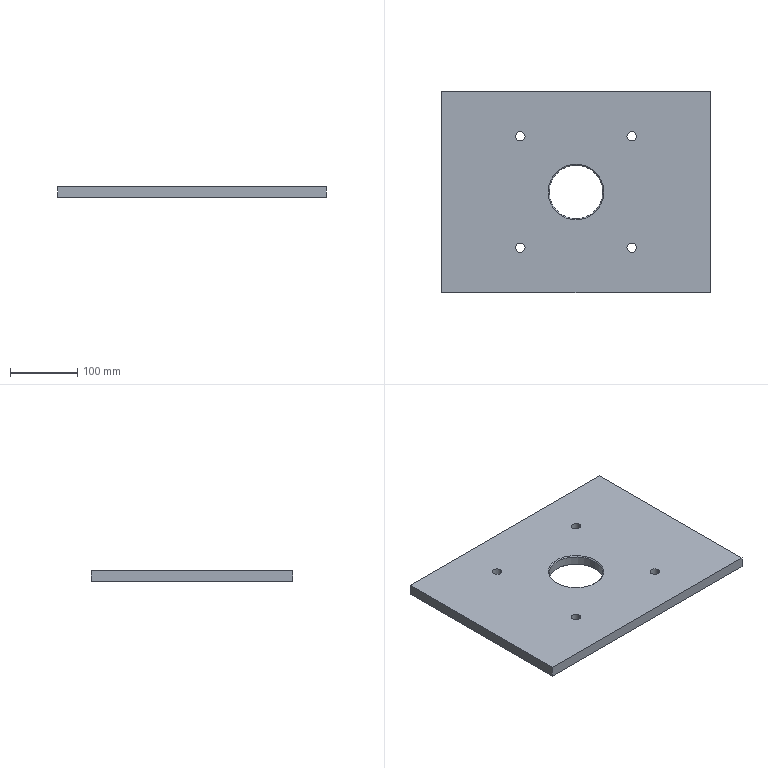Part | STEP file | 04-Base plate | 1 solid | 20 faces | box 400 x 300 x 16 mm | volume 1829151 mm3 | cylinder 10 | plane 6 | cone 4 | commonest cylinder face diameters 14 x8 80 x2
STEP:
#1=CARTESIAN_POINT('',(0.,0.,0.));
#2=DIRECTION('',(0.,0.,1.));
#3=DIRECTION('',(1.,0.,0.));
#4=AXIS2_PLACEMENT_3D('',#1,#2,#3);
#5=CARTESIAN_POINT('',(240.,-150.,14.5));
#6=VERTEX_POINT('',#5);
#7=CARTESIAN_POINT('',(241.5,-150.,16.));
#8=VERTEX_POINT('',#7);
#9=CARTESIAN_POINT('',(240.,-150.,14.5));
#10=DIRECTION('',(0.7071,0.,0.7071));
#11=VECTOR('',#10,1.);
#12=LINE('',#9,#11);
#13=CARTESIAN_POINT('',(200.,-150.,14.5));
#14=DIRECTION('',(0.,0.,1.));
#15=DIRECTION('',(1.,0.,0.));
#16=AXIS2_PLACEMENT_3D('',#13,#14,#15);
#17=CONICAL_SURFACE('',#16,40.,0.7854);
#18=CARTESIAN_POINT('',(6.283,0.));
#19=DIRECTION('',(0.,1.));
#20=VECTOR('',#19,1.);
#21=LINE('',#18,#20);
#22=(GEOMETRIC_REPRESENTATION_CONTEXT(2)PARAMETRIC_REPRESENTATION_CONTEXT()REPRESENTATION_CONTEXT('',''));
#23=DEFINITIONAL_REPRESENTATION('',(#21),#22);
#24=PCURVE('',#17,#23);
#25=CARTESIAN_POINT('',(200.,-150.,14.5));
#26=DIRECTION('',(0.,0.,1.));
#27=DIRECTION('',(1.,0.,0.));
#28=AXIS2_PLACEMENT_3D('',#25,#26,#27);
#29=CONICAL_SURFACE('',#28,40.,0.7854);
#30=CARTESIAN_POINT('',(0.,0.));
#31=DIRECTION('',(0.,1.));
#32=VECTOR('',#31,1.);
#33=LINE('',#30,#32);
#34=(GEOMETRIC_REPRESENTATION_CONTEXT(2)PARAMETRIC_REPRESENTATION_CONTEXT()REPRESENTATION_CONTEXT('',''));
#35=DEFINITIONAL_REPRESENTATION('',(#33),#34);
#36=PCURVE('',#29,#35);
#37=SURFACE_CURVE('',#12,(#24,#36),.PCURVE_S1.);
#38=EDGE_CURVE('',#6,#8,#37,.T.);
#39=ORIENTED_EDGE('',*,*,#38,.T.);
#40=CARTESIAN_POINT('',(158.5,-150.,16.));
#41=VERTEX_POINT('',#40);
#42=CARTESIAN_POINT('',(200.,-150.,16.));
#43=DIRECTION('',(0.,0.,-1.));
#44=DIRECTION('',(1.,0.,0.));
#45=AXIS2_PLACEMENT_3D('',#42,#43,#44);
#46=CIRCLE('',#45,41.5);
#47=CARTESIAN_POINT('',(6.283,1.5));
#48=DIRECTION('',(-1.,0.));
#49=VECTOR('',#48,1.);
#50=LINE('',#47,#49);
#51=(GEOMETRIC_REPRESENTATION_CONTEXT(2)PARAMETRIC_REPRESENTATION_CONTEXT()REPRESENTATION_CONTEXT('',''));
#52=DEFINITIONAL_REPRESENTATION('',(#50),#51);
#53=PCURVE('',#17,#52);
#54=CARTESIAN_POINT('',(0.,0.,16.));
#55=DIRECTION('',(0.,0.,1.));
#56=DIRECTION('',(1.,0.,0.));
#57=AXIS2_PLACEMENT_3D('',#54,#55,#56);
#58=PLANE('',#57);
#59=CARTESIAN_POINT('',(241.5,-150.));
#60=CARTESIAN_POINT('',(241.5,-221.88));
#61=CARTESIAN_POINT('',(179.25,-185.94));
#62=CARTESIAN_POINT('',(117.,-150.));
#63=CARTESIAN_POINT('',(179.25,-114.06));
#64=CARTESIAN_POINT('',(241.5,-78.12));
#65=CARTESIAN_POINT('',(241.5,-150.));
#66=(BOUNDED_CURVE()B_SPLINE_CURVE(2,(#59,#60,#61,#62,#63,#64,#65),.UNSPECIFIED.,.T.,.F.)B_SPLINE_CURVE_WITH_KNOTS((1,2,2,2,2,1),(-2.094,0.,2.094,4.189,6.283,8.378),.UNSPECIFIED.)CURVE()GEOMETRIC_REPRESENTATION_ITEM()RATIONAL_B_SPLINE_CURVE((1.,0.5,1.,0.5,1.,0.5,1.))REPRESENTATION_ITEM(''));
#67=(GEOMETRIC_REPRESENTATION_CONTEXT(2)PARAMETRIC_REPRESENTATION_CONTEXT()REPRESENTATION_CONTEXT('',''));
#68=DEFINITIONAL_REPRESENTATION('',(#66),#67);
#69=PCURVE('',#58,#68);
#70=SURFACE_CURVE('',#46,(#53,#69),.PCURVE_S1.);
#71=EDGE_CURVE('',#8,#41,#70,.T.);
#72=ORIENTED_EDGE('',*,*,#71,.T.);
#73=CARTESIAN_POINT('',(160.,-150.,14.5));
#74=VERTEX_POINT('',#73);
#75=CARTESIAN_POINT('',(160.,-150.,14.5));
#76=DIRECTION('',(-0.7071,0.,0.7071));
#77=VECTOR('',#76,1.);
#78=LINE('',#75,#77);
#79=CARTESIAN_POINT('',(3.142,0.));
#80=DIRECTION('',(0.,1.));
#81=VECTOR('',#80,1.);
#82=LINE('',#79,#81);
#83=(GEOMETRIC_REPRESENTATION_CONTEXT(2)PARAMETRIC_REPRESENTATION_CONTEXT()REPRESENTATION_CONTEXT('',''));
#84=DEFINITIONAL_REPRESENTATION('',(#82),#83);
#85=PCURVE('',#17,#84);
#86=CARTESIAN_POINT('',(3.142,0.));
#87=DIRECTION('',(0.,1.));
#88=VECTOR('',#87,1.);
#89=LINE('',#86,#88);
#90=(GEOMETRIC_REPRESENTATION_CONTEXT(2)PARAMETRIC_REPRESENTATION_CONTEXT()REPRESENTATION_CONTEXT('',''));
#91=DEFINITIONAL_REPRESENTATION('',(#89),#90);
#92=PCURVE('',#29,#91);
#93=SURFACE_CURVE('',#78,(#85,#92),.PCURVE_S1.);
#94=EDGE_CURVE('',#74,#41,#93,.T.);
#95=ORIENTED_EDGE('',*,*,#94,.F.);
#96=CARTESIAN_POINT('',(200.,-150.,14.5));
#97=DIRECTION('',(0.,0.,1.));
#98=DIRECTION('',(1.,0.,0.));
#99=AXIS2_PLACEMENT_3D('',#96,#97,#98);
#100=CIRCLE('',#99,40.);
#101=CARTESIAN_POINT('',(0.,0.));
#102=DIRECTION('',(1.,0.));
#103=VECTOR('',#102,1.);
#104=LINE('',#101,#103);
#105=(GEOMETRIC_REPRESENTATION_CONTEXT(2)PARAMETRIC_REPRESENTATION_CONTEXT()REPRESENTATION_CONTEXT('',''));
#106=DEFINITIONAL_REPRESENTATION('',(#104),#105);
#107=PCURVE('',#17,#106);
#108=CARTESIAN_POINT('',(200.,-150.,16.));
#109=DIRECTION('',(0.,0.,-1.));
#110=DIRECTION('',(-1.,0.,0.));
#111=AXIS2_PLACEMENT_3D('',#108,#109,#110);
#112=CYLINDRICAL_SURFACE('',#111,40.);
#113=CARTESIAN_POINT('',(9.425,1.5));
#114=DIRECTION('',(-1.,0.));
#115=VECTOR('',#114,1.);
#116=LINE('',#113,#115);
#117=(GEOMETRIC_REPRESENTATION_CONTEXT(2)PARAMETRIC_REPRESENTATION_CONTEXT()REPRESENTATION_CONTEXT('',''));
#118=DEFINITIONAL_REPRESENTATION('',(#116),#117);
#119=PCURVE('',#112,#118);
#120=SURFACE_CURVE('',#100,(#107,#119),.PCURVE_S1.);
#121=EDGE_CURVE('',#74,#6,#120,.T.);
#122=ORIENTED_EDGE('',*,*,#121,.T.);
#123=EDGE_LOOP('',(#39,#72,#95,#122));
#124=FACE_BOUND('',#123,.F.);
#125=ADVANCED_FACE('',(#124),#17,.F.);
#126=CARTESIAN_POINT('',(160.,-150.,1.5));
#127=VERTEX_POINT('',#126);
#128=CARTESIAN_POINT('',(158.5,-150.,0.));
#129=VERTEX_POINT('',#128);
#130=CARTESIAN_POINT('',(158.5,-150.,0.));
#131=DIRECTION('',(-0.7071,0.,-0.7071));
#132=VECTOR('',#131,1.);
#133=LINE('',#130,#132);
#134=CARTESIAN_POINT('',(200.,-150.,0.));
#135=DIRECTION('',(0.,0.,-1.));
#136=DIRECTION('',(-1.,0.,0.));
#137=AXIS2_PLACEMENT_3D('',#134,#135,#136);
#138=CONICAL_SURFACE('',#137,41.5,0.7854);
#139=CARTESIAN_POINT('',(6.283,0.));
#140=DIRECTION('',(0.,1.));
#141=VECTOR('',#140,1.);
#142=LINE('',#139,#141);
#143=(GEOMETRIC_REPRESENTATION_CONTEXT(2)PARAMETRIC_REPRESENTATION_CONTEXT()REPRESENTATION_CONTEXT('',''));
#144=DEFINITIONAL_REPRESENTATION('',(#142),#143);
#145=PCURVE('',#138,#144);
#146=CARTESIAN_POINT('',(200.,-150.,0.));
#147=DIRECTION('',(0.,0.,-1.));
#148=DIRECTION('',(-1.,0.,0.));
#149=AXIS2_PLACEMENT_3D('',#146,#147,#148);
#150=CONICAL_SURFACE('',#149,41.5,0.7854);
#151=CARTESIAN_POINT('',(0.,0.));
#152=DIRECTION('',(0.,1.));
#153=VECTOR('',#152,1.);
#154=LINE('',#151,#153);
#155=(GEOMETRIC_REPRESENTATION_CONTEXT(2)PARAMETRIC_REPRESENTATION_CONTEXT()REPRESENTATION_CONTEXT('',''));
#156=DEFINITIONAL_REPRESENTATION('',(#154),#155);
#157=PCURVE('',#150,#156);
#158=SURFACE_CURVE('',#133,(#145,#157),.PCURVE_S1.);
#159=EDGE_CURVE('',#127,#129,#158,.T.);
#160=ORIENTED_EDGE('',*,*,#159,.T.);
#161=CARTESIAN_POINT('',(241.5,-150.,0.));
#162=VERTEX_POINT('',#161);
#163=CARTESIAN_POINT('',(200.,-150.,0.));
#164=DIRECTION('',(0.,0.,1.));
#165=DIRECTION('',(1.,0.,0.));
#166=AXIS2_PLACEMENT_3D('',#163,#164,#165);
#167=CIRCLE('',#166,41.5);
#168=CARTESIAN_POINT('',(9.425,0.));
#169=DIRECTION('',(-1.,0.));
#170=VECTOR('',#169,1.);
#171=LINE('',#168,#170);
#172=(GEOMETRIC_REPRESENTATION_CONTEXT(2)PARAMETRIC_REPRESENTATION_CONTEXT()REPRESENTATION_CONTEXT('',''));
#173=DEFINITIONAL_REPRESENTATION('',(#171),#172);
#174=PCURVE('',#138,#173);
#175=CARTESIAN_POINT('',(0.,0.,0.));
#176=DIRECTION('',(0.,0.,1.));
#177=DIRECTION('',(1.,0.,0.));
#178=AXIS2_PLACEMENT_3D('',#175,#176,#177);
#179=PLANE('',#178);
#180=CARTESIAN_POINT('',(200.,-150.));
#181=DIRECTION('',(1.,0.));
#182=AXIS2_PLACEMENT_2D('',#180,#181);
#183=CIRCLE('',#182,41.5);
#184=(GEOMETRIC_REPRESENTATION_CONTEXT(2)PARAMETRIC_REPRESENTATION_CONTEXT()REPRESENTATION_CONTEXT('',''));
#185=DEFINITIONAL_REPRESENTATION('',(#183),#184);
#186=PCURVE('',#179,#185);
#187=SURFACE_CURVE('',#167,(#174,#186),.PCURVE_S1.);
#188=EDGE_CURVE('',#129,#162,#187,.T.);
#189=ORIENTED_EDGE('',*,*,#188,.T.);
#190=CARTESIAN_POINT('',(240.,-150.,1.5));
#191=VERTEX_POINT('',#190);
#192=CARTESIAN_POINT('',(241.5,-150.,0.));
#193=DIRECTION('',(0.7071,0.,-0.7071));
#194=VECTOR('',#193,1.);
#195=LINE('',#192,#194);
#196=CARTESIAN_POINT('',(3.142,0.));
#197=DIRECTION('',(0.,1.));
#198=VECTOR('',#197,1.);
#199=LINE('',#196,#198);
#200=(GEOMETRIC_REPRESENTATION_CONTEXT(2)PARAMETRIC_REPRESENTATION_CONTEXT()REPRESENTATION_CONTEXT('',''));
#201=DEFINITIONAL_REPRESENTATION('',(#199),#200);
#202=PCURVE('',#138,#201);
#203=CARTESIAN_POINT('',(3.142,0.));
#204=DIRECTION('',(0.,1.));
#205=VECTOR('',#204,1.);
#206=LINE('',#203,#205);
#207=(GEOMETRIC_REPRESENTATION_CONTEXT(2)PARAMETRIC_REPRESENTATION_CONTEXT()REPRESENTATION_CONTEXT('',''));
#208=DEFINITIONAL_REPRESENTATION('',(#206),#207);
#209=PCURVE('',#150,#208);
#210=SURFACE_CURVE('',#195,(#202,#209),.PCURVE_S1.);
#211=EDGE_CURVE('',#191,#162,#210,.T.);
#212=ORIENTED_EDGE('',*,*,#211,.F.);
#213=CARTESIAN_POINT('',(200.,-150.,1.5));
#214=DIRECTION('',(0.,0.,-1.));
#215=DIRECTION('',(1.,0.,0.));
#216=AXIS2_PLACEMENT_3D('',#213,#214,#215);
#217=CIRCLE('',#216,40.);
#218=CARTESIAN_POINT('',(3.142,-1.5));
#219=DIRECTION('',(1.,0.));
#220=VECTOR('',#219,1.);
#221=LINE('',#218,#220);
#222=(GEOMETRIC_REPRESENTATION_CONTEXT(2)PARAMETRIC_REPRESENTATION_CONTEXT()REPRESENTATION_CONTEXT('',''));
#223=DEFINITIONAL_REPRESENTATION('',(#221),#222);
#224=PCURVE('',#138,#223);
#225=CARTESIAN_POINT('',(3.142,14.5));
#226=DIRECTION('',(1.,0.));
#227=VECTOR('',#226,1.);
#228=LINE('',#225,#227);
#229=(GEOMETRIC_REPRESENTATION_CONTEXT(2)PARAMETRIC_REPRESENTATION_CONTEXT()REPRESENTATION_CONTEXT('',''));
#230=DEFINITIONAL_REPRESENTATION('',(#228),#229);
#231=PCURVE('',#112,#230);
#232=SURFACE_CURVE('',#217,(#224,#231),.PCURVE_S1.);
#233=EDGE_CURVE('',#191,#127,#232,.T.);
#234=ORIENTED_EDGE('',*,*,#233,.T.);
#235=EDGE_LOOP('',(#160,#189,#212,#234));
#236=FACE_BOUND('',#235,.F.);
#237=ADVANCED_FACE('',(#236),#138,.F.);
#238=CARTESIAN_POINT('',(124.,-67.,0.));
#239=VERTEX_POINT('',#238);
#240=CARTESIAN_POINT('',(124.,-67.,16.));
#241=VERTEX_POINT('',#240);
#242=CARTESIAN_POINT('',(124.,-67.,16.));
#243=DIRECTION('',(0.,0.,1.));
#244=VECTOR('',#243,1.);
#245=LINE('',#242,#244);
#246=CARTESIAN_POINT('',(117.,-67.,16.));
#247=DIRECTION('',(0.,0.,1.));
#248=DIRECTION('',(1.,0.,0.));
#249=AXIS2_PLACEMENT_3D('',#246,#247,#248);
#250=CYLINDRICAL_SURFACE('',#249,7.);
#251=CARTESIAN_POINT('',(6.283,0.));
#252=DIRECTION('',(0.,1.));
#253=VECTOR('',#252,1.);
#254=LINE('',#251,#253);
#255=(GEOMETRIC_REPRESENTATION_CONTEXT(2)PARAMETRIC_REPRESENTATION_CONTEXT()REPRESENTATION_CONTEXT('',''));
#256=DEFINITIONAL_REPRESENTATION('',(#254),#255);
#257=PCURVE('',#250,#256);
#258=CARTESIAN_POINT('',(117.,-67.,16.));
#259=DIRECTION('',(0.,0.,1.));
#260=DIRECTION('',(1.,0.,0.));
#261=AXIS2_PLACEMENT_3D('',#258,#259,#260);
#262=CYLINDRICAL_SURFACE('',#261,7.);
#263=CARTESIAN_POINT('',(0.,0.));
#264=DIRECTION('',(0.,1.));
#265=VECTOR('',#264,1.);
#266=LINE('',#263,#265);
#267=(GEOMETRIC_REPRESENTATION_CONTEXT(2)PARAMETRIC_REPRESENTATION_CONTEXT()REPRESENTATION_CONTEXT('',''));
#268=DEFINITIONAL_REPRESENTATION('',(#266),#267);
#269=PCURVE('',#262,#268);
#270=SURFACE_CURVE('',#245,(#257,#269),.PCURVE_S1.);
#271=EDGE_CURVE('',#239,#241,#270,.T.);
#272=ORIENTED_EDGE('',*,*,#271,.T.);
#273=CARTESIAN_POINT('',(110.,-67.,16.));
#274=VERTEX_POINT('',#273);
#275=CARTESIAN_POINT('',(117.,-67.,16.));
#276=DIRECTION('',(0.,0.,1.));
#277=DIRECTION('',(1.,0.,0.));
#278=AXIS2_PLACEMENT_3D('',#275,#276,#277);
#279=CIRCLE('',#278,7.);
#280=CARTESIAN_POINT('',(0.,0.));
#281=DIRECTION('',(1.,0.));
#282=VECTOR('',#281,1.);
#283=LINE('',#280,#282);
#284=(GEOMETRIC_REPRESENTATION_CONTEXT(2)PARAMETRIC_REPRESENTATION_CONTEXT()REPRESENTATION_CONTEXT('',''));
#285=DEFINITIONAL_REPRESENTATION('',(#283),#284);
#286=PCURVE('',#250,#285);
#287=CARTESIAN_POINT('',(117.,-67.));
#288=DIRECTION('',(1.,0.));
#289=AXIS2_PLACEMENT_2D('',#287,#288);
#290=CIRCLE('',#289,7.);
#291=(GEOMETRIC_REPRESENTATION_CONTEXT(2)PARAMETRIC_REPRESENTATION_CONTEXT()REPRESENTATION_CONTEXT('',''));
#292=DEFINITIONAL_REPRESENTATION('',(#290),#291);
#293=PCURVE('',#58,#292);
#294=SURFACE_CURVE('',#279,(#286,#293),.PCURVE_S1.);
#295=EDGE_CURVE('',#274,#241,#294,.T.);
#296=ORIENTED_EDGE('',*,*,#295,.F.);
#297=CARTESIAN_POINT('',(110.,-67.,0.));
#298=VERTEX_POINT('',#297);
#299=CARTESIAN_POINT('',(110.,-67.,16.));
#300=DIRECTION('',(0.,0.,1.));
#301=VECTOR('',#300,1.);
#302=LINE('',#299,#301);
#303=CARTESIAN_POINT('',(3.142,0.));
#304=DIRECTION('',(0.,1.));
#305=VECTOR('',#304,1.);
#306=LINE('',#303,#305);
#307=(GEOMETRIC_REPRESENTATION_CONTEXT(2)PARAMETRIC_REPRESENTATION_CONTEXT()REPRESENTATION_CONTEXT('',''));
#308=DEFINITIONAL_REPRESENTATION('',(#306),#307);
#309=PCURVE('',#250,#308);
#310=CARTESIAN_POINT('',(3.142,0.));
#311=DIRECTION('',(0.,1.));
#312=VECTOR('',#311,1.);
#313=LINE('',#310,#312);
#314=(GEOMETRIC_REPRESENTATION_CONTEXT(2)PARAMETRIC_REPRESENTATION_CONTEXT()REPRESENTATION_CONTEXT('',''));
#315=DEFINITIONAL_REPRESENTATION('',(#313),#314);
#316=PCURVE('',#262,#315);
#317=SURFACE_CURVE('',#302,(#309,#316),.PCURVE_S1.);
#318=EDGE_CURVE('',#298,#274,#317,.T.);
#319=ORIENTED_EDGE('',*,*,#318,.F.);
#320=CARTESIAN_POINT('',(117.,-67.,0.));
#321=DIRECTION('',(0.,0.,1.));
#322=DIRECTION('',(1.,0.,0.));
#323=AXIS2_PLACEMENT_3D('',#320,#321,#322);
#324=CIRCLE('',#323,7.);
#325=CARTESIAN_POINT('',(0.,-16.));
#326=DIRECTION('',(1.,0.));
#327=VECTOR('',#326,1.);
#328=LINE('',#325,#327);
#329=(GEOMETRIC_REPRESENTATION_CONTEXT(2)PARAMETRIC_REPRESENTATION_CONTEXT()REPRESENTATION_CONTEXT('',''));
#330=DEFINITIONAL_REPRESENTATION('',(#328),#329);
#331=PCURVE('',#250,#330);
#332=CARTESIAN_POINT('',(117.,-67.));
#333=DIRECTION('',(1.,0.));
#334=AXIS2_PLACEMENT_2D('',#332,#333);
#335=CIRCLE('',#334,7.);
#336=(GEOMETRIC_REPRESENTATION_CONTEXT(2)PARAMETRIC_REPRESENTATION_CONTEXT()REPRESENTATION_CONTEXT('',''));
#337=DEFINITIONAL_REPRESENTATION('',(#335),#336);
#338=PCURVE('',#179,#337);
#339=SURFACE_CURVE('',#324,(#331,#338),.PCURVE_S1.);
#340=EDGE_CURVE('',#298,#239,#339,.T.);
#341=ORIENTED_EDGE('',*,*,#340,.T.);
#342=EDGE_LOOP('',(#272,#296,#319,#341));
#343=FACE_BOUND('',#342,.F.);
#344=ADVANCED_FACE('',(#343),#250,.F.);
#345=CARTESIAN_POINT('',(290.,-67.,0.));
#346=VERTEX_POINT('',#345);
#347=CARTESIAN_POINT('',(290.,-67.,16.));
#348=VERTEX_POINT('',#347);
#349=CARTESIAN_POINT('',(290.,-67.,16.));
#350=DIRECTION('',(0.,0.,1.));
#351=VECTOR('',#350,1.);
#352=LINE('',#349,#351);
#353=CARTESIAN_POINT('',(283.,-67.,16.));
#354=DIRECTION('',(0.,0.,1.));
#355=DIRECTION('',(1.,0.,0.));
#356=AXIS2_PLACEMENT_3D('',#353,#354,#355);
#357=CYLINDRICAL_SURFACE('',#356,7.);
#358=CARTESIAN_POINT('',(6.283,0.));
#359=DIRECTION('',(0.,1.));
#360=VECTOR('',#359,1.);
#361=LINE('',#358,#360);
#362=(GEOMETRIC_REPRESENTATION_CONTEXT(2)PARAMETRIC_REPRESENTATION_CONTEXT()REPRESENTATION_CONTEXT('',''));
#363=DEFINITIONAL_REPRESENTATION('',(#361),#362);
#364=PCURVE('',#357,#363);
#365=CARTESIAN_POINT('',(283.,-67.,16.));
#366=DIRECTION('',(0.,0.,1.));
#367=DIRECTION('',(1.,0.,0.));
#368=AXIS2_PLACEMENT_3D('',#365,#366,#367);
#369=CYLINDRICAL_SURFACE('',#368,7.);
#370=CARTESIAN_POINT('',(0.,0.));
#371=DIRECTION('',(0.,1.));
#372=VECTOR('',#371,1.);
#373=LINE('',#370,#372);
#374=(GEOMETRIC_REPRESENTATION_CONTEXT(2)PARAMETRIC_REPRESENTATION_CONTEXT()REPRESENTATION_CONTEXT('',''));
#375=DEFINITIONAL_REPRESENTATION('',(#373),#374);
#376=PCURVE('',#369,#375);
#377=SURFACE_CURVE('',#352,(#364,#376),.PCURVE_S1.);
#378=EDGE_CURVE('',#346,#348,#377,.T.);
#379=ORIENTED_EDGE('',*,*,#378,.T.);
#380=CARTESIAN_POINT('',(276.,-67.,16.));
#381=VERTEX_POINT('',#380);
#382=CARTESIAN_POINT('',(283.,-67.,16.));
#383=DIRECTION('',(0.,0.,1.));
#384=DIRECTION('',(1.,0.,0.));
#385=AXIS2_PLACEMENT_3D('',#382,#383,#384);
#386=CIRCLE('',#385,7.);
#387=CARTESIAN_POINT('',(0.,0.));
#388=DIRECTION('',(1.,0.));
#389=VECTOR('',#388,1.);
#390=LINE('',#387,#389);
#391=(GEOMETRIC_REPRESENTATION_CONTEXT(2)PARAMETRIC_REPRESENTATION_CONTEXT()REPRESENTATION_CONTEXT('',''));
#392=DEFINITIONAL_REPRESENTATION('',(#390),#391);
#393=PCURVE('',#357,#392);
#394=CARTESIAN_POINT('',(283.,-67.));
#395=DIRECTION('',(1.,0.));
#396=AXIS2_PLACEMENT_2D('',#394,#395);
#397=CIRCLE('',#396,7.);
#398=(GEOMETRIC_REPRESENTATION_CONTEXT(2)PARAMETRIC_REPRESENTATION_CONTEXT()REPRESENTATION_CONTEXT('',''));
#399=DEFINITIONAL_REPRESENTATION('',(#397),#398);
#400=PCURVE('',#58,#399);
#401=SURFACE_CURVE('',#386,(#393,#400),.PCURVE_S1.);
#402=EDGE_CURVE('',#381,#348,#401,.T.);
#403=ORIENTED_EDGE('',*,*,#402,.F.);
#404=CARTESIAN_POINT('',(276.,-67.,0.));
#405=VERTEX_POINT('',#404);
#406=CARTESIAN_POINT('',(276.,-67.,16.));
#407=DIRECTION('',(0.,0.,1.));
#408=VECTOR('',#407,1.);
#409=LINE('',#406,#408);
#410=CARTESIAN_POINT('',(3.142,0.));
#411=DIRECTION('',(0.,1.));
#412=VECTOR('',#411,1.);
#413=LINE('',#410,#412);
#414=(GEOMETRIC_REPRESENTATION_CONTEXT(2)PARAMETRIC_REPRESENTATION_CONTEXT()REPRESENTATION_CONTEXT('',''));
#415=DEFINITIONAL_REPRESENTATION('',(#413),#414);
#416=PCURVE('',#357,#415);
#417=CARTESIAN_POINT('',(3.142,0.));
#418=DIRECTION('',(0.,1.));
#419=VECTOR('',#418,1.);
#420=LINE('',#417,#419);
#421=(GEOMETRIC_REPRESENTATION_CONTEXT(2)PARAMETRIC_REPRESENTATION_CONTEXT()REPRESENTATION_CONTEXT('',''));
#422=DEFINITIONAL_REPRESENTATION('',(#420),#421);
#423=PCURVE('',#369,#422);
#424=SURFACE_CURVE('',#409,(#416,#423),.PCURVE_S1.);
#425=EDGE_CURVE('',#405,#381,#424,.T.);
#426=ORIENTED_EDGE('',*,*,#425,.F.);
#427=CARTESIAN_POINT('',(283.,-67.,0.));
#428=DIRECTION('',(0.,0.,1.));
#429=DIRECTION('',(1.,0.,0.));
#430=AXIS2_PLACEMENT_3D('',#427,#428,#429);
#431=CIRCLE('',#430,7.);
#432=CARTESIAN_POINT('',(0.,-16.));
#433=DIRECTION('',(1.,0.));
#434=VECTOR('',#433,1.);
#435=LINE('',#432,#434);
#436=(GEOMETRIC_REPRESENTATION_CONTEXT(2)PARAMETRIC_REPRESENTATION_CONTEXT()REPRESENTATION_CONTEXT('',''));
#437=DEFINITIONAL_REPRESENTATION('',(#435),#436);
#438=PCURVE('',#357,#437);
#439=CARTESIAN_POINT('',(283.,-67.));
#440=DIRECTION('',(1.,0.));
#441=AXIS2_PLACEMENT_2D('',#439,#440);
#442=CIRCLE('',#441,7.);
#443=(GEOMETRIC_REPRESENTATION_CONTEXT(2)PARAMETRIC_REPRESENTATION_CONTEXT()REPRESENTATION_CONTEXT('',''));
#444=DEFINITIONAL_REPRESENTATION('',(#442),#443);
#445=PCURVE('',#179,#444);
#446=SURFACE_CURVE('',#431,(#438,#445),.PCURVE_S1.);
#447=EDGE_CURVE('',#405,#346,#446,.T.);
#448=ORIENTED_EDGE('',*,*,#447,.T.);
#449=EDGE_LOOP('',(#379,#403,#426,#448));
#450=FACE_BOUND('',#449,.F.);
#451=ADVANCED_FACE('',(#450),#357,.F.);
#452=CARTESIAN_POINT('',(290.,-233.,0.));
#453=VERTEX_POINT('',#452);
#454=CARTESIAN_POINT('',(290.,-233.,16.));
#455=VERTEX_POINT('',#454);
#456=CARTESIAN_POINT('',(290.,-233.,16.));
#457=DIRECTION('',(0.,0.,1.));
#458=VECTOR('',#457,1.);
#459=LINE('',#456,#458);
#460=CARTESIAN_POINT('',(283.,-233.,16.));
#461=DIRECTION('',(0.,0.,1.));
#462=DIRECTION('',(1.,0.,0.));
#463=AXIS2_PLACEMENT_3D('',#460,#461,#462);
#464=CYLINDRICAL_SURFACE('',#463,7.);
#465=CARTESIAN_POINT('',(6.283,0.));
#466=DIRECTION('',(0.,1.));
#467=VECTOR('',#466,1.);
#468=LINE('',#465,#467);
#469=(GEOMETRIC_REPRESENTATION_CONTEXT(2)PARAMETRIC_REPRESENTATION_CONTEXT()REPRESENTATION_CONTEXT('',''));
#470=DEFINITIONAL_REPRESENTATION('',(#468),#469);
#471=PCURVE('',#464,#470);
#472=CARTESIAN_POINT('',(283.,-233.,16.));
#473=DIRECTION('',(0.,0.,1.));
#474=DIRECTION('',(1.,0.,0.));
#475=AXIS2_PLACEMENT_3D('',#472,#473,#474);
#476=CYLINDRICAL_SURFACE('',#475,7.);
#477=CARTESIAN_POINT('',(0.,0.));
#478=DIRECTION('',(0.,1.));
#479=VECTOR('',#478,1.);
#480=LINE('',#477,#479);
#481=(GEOMETRIC_REPRESENTATION_CONTEXT(2)PARAMETRIC_REPRESENTATION_CONTEXT()REPRESENTATION_CONTEXT('',''));
#482=DEFINITIONAL_REPRESENTATION('',(#480),#481);
#483=PCURVE('',#476,#482);
#484=SURFACE_CURVE('',#459,(#471,#483),.PCURVE_S1.);
#485=EDGE_CURVE('',#453,#455,#484,.T.);
#486=ORIENTED_EDGE('',*,*,#485,.T.);
#487=CARTESIAN_POINT('',(276.,-233.,16.));
#488=VERTEX_POINT('',#487);
#489=CARTESIAN_POINT('',(283.,-233.,16.));
#490=DIRECTION('',(0.,0.,1.));
#491=DIRECTION('',(1.,0.,0.));
#492=AXIS2_PLACEMENT_3D('',#489,#490,#491);
#493=CIRCLE('',#492,7.);
#494=CARTESIAN_POINT('',(0.,0.));
#495=DIRECTION('',(1.,0.));
#496=VECTOR('',#495,1.);
#497=LINE('',#494,#496);
#498=(GEOMETRIC_REPRESENTATION_CONTEXT(2)PARAMETRIC_REPRESENTATION_CONTEXT()REPRESENTATION_CONTEXT('',''));
#499=DEFINITIONAL_REPRESENTATION('',(#497),#498);
#500=PCURVE('',#464,#499);
#501=CARTESIAN_POINT('',(283.,-233.));
#502=DIRECTION('',(1.,0.));
#503=AXIS2_PLACEMENT_2D('',#501,#502);
#504=CIRCLE('',#503,7.);
#505=(GEOMETRIC_REPRESENTATION_CONTEXT(2)PARAMETRIC_REPRESENTATION_CONTEXT()REPRESENTATION_CONTEXT('',''));
#506=DEFINITIONAL_REPRESENTATION('',(#504),#505);
#507=PCURVE('',#58,#506);
#508=SURFACE_CURVE('',#493,(#500,#507),.PCURVE_S1.);
#509=EDGE_CURVE('',#488,#455,#508,.T.);
#510=ORIENTED_EDGE('',*,*,#509,.F.);
#511=CARTESIAN_POINT('',(276.,-233.,0.));
#512=VERTEX_POINT('',#511);
#513=CARTESIAN_POINT('',(276.,-233.,16.));
#514=DIRECTION('',(0.,0.,1.));
#515=VECTOR('',#514,1.);
#516=LINE('',#513,#515);
#517=CARTESIAN_POINT('',(3.142,0.));
#518=DIRECTION('',(0.,1.));
#519=VECTOR('',#518,1.);
#520=LINE('',#517,#519);
#521=(GEOMETRIC_REPRESENTATION_CONTEXT(2)PARAMETRIC_REPRESENTATION_CONTEXT()REPRESENTATION_CONTEXT('',''));
#522=DEFINITIONAL_REPRESENTATION('',(#520),#521);
#523=PCURVE('',#464,#522);
#524=CARTESIAN_POINT('',(3.142,0.));
#525=DIRECTION('',(0.,1.));
#526=VECTOR('',#525,1.);
#527=LINE('',#524,#526);
#528=(GEOMETRIC_REPRESENTATION_CONTEXT(2)PARAMETRIC_REPRESENTATION_CONTEXT()REPRESENTATION_CONTEXT('',''));
#529=DEFINITIONAL_REPRESENTATION('',(#527),#528);
#530=PCURVE('',#476,#529);
#531=SURFACE_CURVE('',#516,(#523,#530),.PCURVE_S1.);
#532=EDGE_CURVE('',#512,#488,#531,.T.);
#533=ORIENTED_EDGE('',*,*,#532,.F.);
#534=CARTESIAN_POINT('',(283.,-233.,0.));
#535=DIRECTION('',(0.,0.,1.));
#536=DIRECTION('',(1.,0.,0.));
#537=AXIS2_PLACEMENT_3D('',#534,#535,#536);
#538=CIRCLE('',#537,7.);
#539=CARTESIAN_POINT('',(0.,-16.));
#540=DIRECTION('',(1.,0.));
#541=VECTOR('',#540,1.);
#542=LINE('',#539,#541);
#543=(GEOMETRIC_REPRESENTATION_CONTEXT(2)PARAMETRIC_REPRESENTATION_CONTEXT()REPRESENTATION_CONTEXT('',''));
#544=DEFINITIONAL_REPRESENTATION('',(#542),#543);
#545=PCURVE('',#464,#544);
#546=CARTESIAN_POINT('',(283.,-233.));
#547=DIRECTION('',(1.,0.));
#548=AXIS2_PLACEMENT_2D('',#546,#547);
#549=CIRCLE('',#548,7.);
#550=(GEOMETRIC_REPRESENTATION_CONTEXT(2)PARAMETRIC_REPRESENTATION_CONTEXT()REPRESENTATION_CONTEXT('',''));
#551=DEFINITIONAL_REPRESENTATION('',(#549),#550);
#552=PCURVE('',#179,#551);
#553=SURFACE_CURVE('',#538,(#545,#552),.PCURVE_S1.);
#554=EDGE_CURVE('',#512,#453,#553,.T.);
#555=ORIENTED_EDGE('',*,*,#554,.T.);
#556=EDGE_LOOP('',(#486,#510,#533,#555));
#557=FACE_BOUND('',#556,.F.);
#558=ADVANCED_FACE('',(#557),#464,.F.);
#559=CARTESIAN_POINT('',(124.,-233.,0.));
#560=VERTEX_POINT('',#559);
#561=CARTESIAN_POINT('',(124.,-233.,16.));
#562=VERTEX_POINT('',#561);
#563=CARTESIAN_POINT('',(124.,-233.,16.));
#564=DIRECTION('',(0.,0.,1.));
#565=VECTOR('',#564,1.);
#566=LINE('',#563,#565);
#567=CARTESIAN_POINT('',(117.,-233.,16.));
#568=DIRECTION('',(0.,0.,1.));
#569=DIRECTION('',(1.,0.,0.));
#570=AXIS2_PLACEMENT_3D('',#567,#568,#569);
#571=CYLINDRICAL_SURFACE('',#570,7.);
#572=CARTESIAN_POINT('',(6.283,0.));
#573=DIRECTION('',(0.,1.));
#574=VECTOR('',#573,1.);
#575=LINE('',#572,#574);
#576=(GEOMETRIC_REPRESENTATION_CONTEXT(2)PARAMETRIC_REPRESENTATION_CONTEXT()REPRESENTATION_CONTEXT('',''));
#577=DEFINITIONAL_REPRESENTATION('',(#575),#576);
#578=PCURVE('',#571,#577);
#579=CARTESIAN_POINT('',(117.,-233.,16.));
#580=DIRECTION('',(0.,0.,1.));
#581=DIRECTION('',(1.,0.,0.));
#582=AXIS2_PLACEMENT_3D('',#579,#580,#581);
#583=CYLINDRICAL_SURFACE('',#582,7.);
#584=CARTESIAN_POINT('',(0.,0.));
#585=DIRECTION('',(0.,1.));
#586=VECTOR('',#585,1.);
#587=LINE('',#584,#586);
#588=(GEOMETRIC_REPRESENTATION_CONTEXT(2)PARAMETRIC_REPRESENTATION_CONTEXT()REPRESENTATION_CONTEXT('',''));
#589=DEFINITIONAL_REPRESENTATION('',(#587),#588);
#590=PCURVE('',#583,#589);
#591=SURFACE_CURVE('',#566,(#578,#590),.PCURVE_S1.);
#592=EDGE_CURVE('',#560,#562,#591,.T.);
#593=ORIENTED_EDGE('',*,*,#592,.T.);
#594=CARTESIAN_POINT('',(110.,-233.,16.));
#595=VERTEX_POINT('',#594);
#596=CARTESIAN_POINT('',(117.,-233.,16.));
#597=DIRECTION('',(0.,0.,1.));
#598=DIRECTION('',(1.,0.,0.));
#599=AXIS2_PLACEMENT_3D('',#596,#597,#598);
#600=CIRCLE('',#599,7.);
#601=CARTESIAN_POINT('',(0.,0.));
#602=DIRECTION('',(1.,0.));
#603=VECTOR('',#602,1.);
#604=LINE('',#601,#603);
#605=(GEOMETRIC_REPRESENTATION_CONTEXT(2)PARAMETRIC_REPRESENTATION_CONTEXT()REPRESENTATION_CONTEXT('',''));
#606=DEFINITIONAL_REPRESENTATION('',(#604),#605);
#607=PCURVE('',#571,#606);
#608=CARTESIAN_POINT('',(117.,-233.));
#609=DIRECTION('',(1.,0.));
#610=AXIS2_PLACEMENT_2D('',#608,#609);
#611=CIRCLE('',#610,7.);
#612=(GEOMETRIC_REPRESENTATION_CONTEXT(2)PARAMETRIC_REPRESENTATION_CONTEXT()REPRESENTATION_CONTEXT('',''));
#613=DEFINITIONAL_REPRESENTATION('',(#611),#612);
#614=PCURVE('',#58,#613);
#615=SURFACE_CURVE('',#600,(#607,#614),.PCURVE_S1.);
#616=EDGE_CURVE('',#595,#562,#615,.T.);
#617=ORIENTED_EDGE('',*,*,#616,.F.);
#618=CARTESIAN_POINT('',(110.,-233.,0.));
#619=VERTEX_POINT('',#618);
#620=CARTESIAN_POINT('',(110.,-233.,16.));
#621=DIRECTION('',(0.,0.,1.));
#622=VECTOR('',#621,1.);
#623=LINE('',#620,#622);
#624=CARTESIAN_POINT('',(3.142,0.));
#625=DIRECTION('',(0.,1.));
#626=VECTOR('',#625,1.);
#627=LINE('',#624,#626);
#628=(GEOMETRIC_REPRESENTATION_CONTEXT(2)PARAMETRIC_REPRESENTATION_CONTEXT()REPRESENTATION_CONTEXT('',''));
#629=DEFINITIONAL_REPRESENTATION('',(#627),#628);
#630=PCURVE('',#571,#629);
#631=CARTESIAN_POINT('',(3.142,0.));
#632=DIRECTION('',(0.,1.));
#633=VECTOR('',#632,1.);
#634=LINE('',#631,#633);
#635=(GEOMETRIC_REPRESENTATION_CONTEXT(2)PARAMETRIC_REPRESENTATION_CONTEXT()REPRESENTATION_CONTEXT('',''));
#636=DEFINITIONAL_REPRESENTATION('',(#634),#635);
#637=PCURVE('',#583,#636);
#638=SURFACE_CURVE('',#623,(#630,#637),.PCURVE_S1.);
#639=EDGE_CURVE('',#619,#595,#638,.T.);
#640=ORIENTED_EDGE('',*,*,#639,.F.);
#641=CARTESIAN_POINT('',(117.,-233.,0.));
#642=DIRECTION('',(0.,0.,1.));
#643=DIRECTION('',(1.,0.,0.));
#644=AXIS2_PLACEMENT_3D('',#641,#642,#643);
#645=CIRCLE('',#644,7.);
#646=CARTESIAN_POINT('',(0.,-16.));
#647=DIRECTION('',(1.,0.));
#648=VECTOR('',#647,1.);
#649=LINE('',#646,#648);
#650=(GEOMETRIC_REPRESENTATION_CONTEXT(2)PARAMETRIC_REPRESENTATION_CONTEXT()REPRESENTATION_CONTEXT('',''));
#651=DEFINITIONAL_REPRESENTATION('',(#649),#650);
#652=PCURVE('',#571,#651);
#653=CARTESIAN_POINT('',(117.,-233.));
#654=DIRECTION('',(1.,0.));
#655=AXIS2_PLACEMENT_2D('',#653,#654);
#656=CIRCLE('',#655,7.);
#657=(GEOMETRIC_REPRESENTATION_CONTEXT(2)PARAMETRIC_REPRESENTATION_CONTEXT()REPRESENTATION_CONTEXT('',''));
#658=DEFINITIONAL_REPRESENTATION('',(#656),#657);
#659=PCURVE('',#179,#658);
#660=SURFACE_CURVE('',#645,(#652,#659),.PCURVE_S1.);
#661=EDGE_CURVE('',#619,#560,#660,.T.);
#662=ORIENTED_EDGE('',*,*,#661,.T.);
#663=EDGE_LOOP('',(#593,#617,#640,#662));
#664=FACE_BOUND('',#663,.F.);
#665=ADVANCED_FACE('',(#664),#571,.F.);
#666=CARTESIAN_POINT('',(160.,-150.,16.));
#667=DIRECTION('',(0.,0.,-1.));
#668=VECTOR('',#667,1.);
#669=LINE('',#666,#668);
#670=CARTESIAN_POINT('',(6.283,0.));
#671=DIRECTION('',(0.,1.));
#672=VECTOR('',#671,1.);
#673=LINE('',#670,#672);
#674=(GEOMETRIC_REPRESENTATION_CONTEXT(2)PARAMETRIC_REPRESENTATION_CONTEXT()REPRESENTATION_CONTEXT('',''));
#675=DEFINITIONAL_REPRESENTATION('',(#673),#674);
#676=PCURVE('',#112,#675);
#677=CARTESIAN_POINT('',(200.,-150.,16.));
#678=DIRECTION('',(0.,0.,-1.));
#679=DIRECTION('',(-1.,0.,0.));
#680=AXIS2_PLACEMENT_3D('',#677,#678,#679);
#681=CYLINDRICAL_SURFACE('',#680,40.);
#682=CARTESIAN_POINT('',(0.,0.));
#683=DIRECTION('',(0.,1.));
#684=VECTOR('',#683,1.);
#685=LINE('',#682,#684);
#686=(GEOMETRIC_REPRESENTATION_CONTEXT(2)PARAMETRIC_REPRESENTATION_CONTEXT()REPRESENTATION_CONTEXT('',''));
#687=DEFINITIONAL_REPRESENTATION('',(#685),#686);
#688=PCURVE('',#681,#687);
#689=SURFACE_CURVE('',#669,(#676,#688),.PCURVE_S1.);
#690=EDGE_CURVE('',#74,#127,#689,.T.);
#691=ORIENTED_EDGE('',*,*,#690,.T.);
#692=ORIENTED_EDGE('',*,*,#233,.F.);
#693=CARTESIAN_POINT('',(240.,-150.,16.));
#694=DIRECTION('',(0.,0.,-1.));
#695=VECTOR('',#694,1.);
#696=LINE('',#693,#695);
#697=CARTESIAN_POINT('',(3.142,0.));
#698=DIRECTION('',(0.,1.));
#699=VECTOR('',#698,1.);
#700=LINE('',#697,#699);
#701=(GEOMETRIC_REPRESENTATION_CONTEXT(2)PARAMETRIC_REPRESENTATION_CONTEXT()REPRESENTATION_CONTEXT('',''));
#702=DEFINITIONAL_REPRESENTATION('',(#700),#701);
#703=PCURVE('',#112,#702);
#704=CARTESIAN_POINT('',(3.142,0.));
#705=DIRECTION('',(0.,1.));
#706=VECTOR('',#705,1.);
#707=LINE('',#704,#706);
#708=(GEOMETRIC_REPRESENTATION_CONTEXT(2)PARAMETRIC_REPRESENTATION_CONTEXT()REPRESENTATION_CONTEXT('',''));
#709=DEFINITIONAL_REPRESENTATION('',(#707),#708);
#710=PCURVE('',#681,#709);
#711=SURFACE_CURVE('',#696,(#703,#710),.PCURVE_S1.);
#712=EDGE_CURVE('',#6,#191,#711,.T.);
#713=ORIENTED_EDGE('',*,*,#712,.F.);
#714=ORIENTED_EDGE('',*,*,#121,.F.);
#715=EDGE_LOOP('',(#691,#692,#713,#714));
#716=FACE_BOUND('',#715,.F.);
#717=ADVANCED_FACE('',(#716),#112,.F.);
#718=ORIENTED_EDGE('',*,*,#71,.T.);
#719=CARTESIAN_POINT('',(200.,-150.,16.));
#720=DIRECTION('',(0.,0.,-1.));
#721=DIRECTION('',(1.,0.,0.));
#722=AXIS2_PLACEMENT_3D('',#719,#720,#721);
#723=CIRCLE('',#722,41.5);
#724=CARTESIAN_POINT('',(241.5,-150.));
#725=CARTESIAN_POINT('',(241.5,-221.88));
#726=CARTESIAN_POINT('',(179.25,-185.94));
#727=CARTESIAN_POINT('',(117.,-150.));
#728=CARTESIAN_POINT('',(179.25,-114.06));
#729=CARTESIAN_POINT('',(241.5,-78.12));
#730=CARTESIAN_POINT('',(241.5,-150.));
#731=(BOUNDED_CURVE()B_SPLINE_CURVE(2,(#724,#725,#726,#727,#728,#729,#730),.UNSPECIFIED.,.T.,.F.)B_SPLINE_CURVE_WITH_KNOTS((1,2,2,2,2,1),(-2.094,0.,2.094,4.189,6.283,8.378),.UNSPECIFIED.)CURVE()GEOMETRIC_REPRESENTATION_ITEM()RATIONAL_B_SPLINE_CURVE((1.,0.5,1.,0.5,1.,0.5,1.))REPRESENTATION_ITEM(''));
#732=(GEOMETRIC_REPRESENTATION_CONTEXT(2)PARAMETRIC_REPRESENTATION_CONTEXT()REPRESENTATION_CONTEXT('',''));
#733=DEFINITIONAL_REPRESENTATION('',(#731),#732);
#734=PCURVE('',#58,#733);
#735=CARTESIAN_POINT('',(6.283,1.5));
#736=DIRECTION('',(-1.,0.));
#737=VECTOR('',#736,1.);
#738=LINE('',#735,#737);
#739=(GEOMETRIC_REPRESENTATION_CONTEXT(2)PARAMETRIC_REPRESENTATION_CONTEXT()REPRESENTATION_CONTEXT('',''));
#740=DEFINITIONAL_REPRESENTATION('',(#738),#739);
#741=PCURVE('',#29,#740);
#742=SURFACE_CURVE('',#723,(#734,#741),.PCURVE_S1.);
#743=EDGE_CURVE('',#41,#8,#742,.T.);
#744=ORIENTED_EDGE('',*,*,#743,.T.);
#745=EDGE_LOOP('',(#718,#744));
#746=FACE_BOUND('',#745,.T.);
#747=CARTESIAN_POINT('',(117.,-67.,16.));
#748=DIRECTION('',(0.,0.,1.));
#749=DIRECTION('',(1.,0.,0.));
#750=AXIS2_PLACEMENT_3D('',#747,#748,#749);
#751=CIRCLE('',#750,7.);
#752=CARTESIAN_POINT('',(117.,-67.));
#753=DIRECTION('',(1.,0.));
#754=AXIS2_PLACEMENT_2D('',#752,#753);
#755=CIRCLE('',#754,7.);
#756=(GEOMETRIC_REPRESENTATION_CONTEXT(2)PARAMETRIC_REPRESENTATION_CONTEXT()REPRESENTATION_CONTEXT('',''));
#757=DEFINITIONAL_REPRESENTATION('',(#755),#756);
#758=PCURVE('',#58,#757);
#759=CARTESIAN_POINT('',(0.,0.));
#760=DIRECTION('',(1.,0.));
#761=VECTOR('',#760,1.);
#762=LINE('',#759,#761);
#763=(GEOMETRIC_REPRESENTATION_CONTEXT(2)PARAMETRIC_REPRESENTATION_CONTEXT()REPRESENTATION_CONTEXT('',''));
#764=DEFINITIONAL_REPRESENTATION('',(#762),#763);
#765=PCURVE('',#262,#764);
#766=SURFACE_CURVE('',#751,(#758,#765),.PCURVE_S1.);
#767=EDGE_CURVE('',#241,#274,#766,.T.);
#768=ORIENTED_EDGE('',*,*,#767,.F.);
#769=ORIENTED_EDGE('',*,*,#295,.F.);
#770=EDGE_LOOP('',(#768,#769));
#771=FACE_BOUND('',#770,.T.);
#772=CARTESIAN_POINT('',(283.,-67.,16.));
#773=DIRECTION('',(0.,0.,1.));
#774=DIRECTION('',(1.,0.,0.));
#775=AXIS2_PLACEMENT_3D('',#772,#773,#774);
#776=CIRCLE('',#775,7.);
#777=CARTESIAN_POINT('',(283.,-67.));
#778=DIRECTION('',(1.,0.));
#779=AXIS2_PLACEMENT_2D('',#777,#778);
#780=CIRCLE('',#779,7.);
#781=(GEOMETRIC_REPRESENTATION_CONTEXT(2)PARAMETRIC_REPRESENTATION_CONTEXT()REPRESENTATION_CONTEXT('',''));
#782=DEFINITIONAL_REPRESENTATION('',(#780),#781);
#783=PCURVE('',#58,#782);
#784=CARTESIAN_POINT('',(0.,0.));
#785=DIRECTION('',(1.,0.));
#786=VECTOR('',#785,1.);
#787=LINE('',#784,#786);
#788=(GEOMETRIC_REPRESENTATION_CONTEXT(2)PARAMETRIC_REPRESENTATION_CONTEXT()REPRESENTATION_CONTEXT('',''));
#789=DEFINITIONAL_REPRESENTATION('',(#787),#788);
#790=PCURVE('',#369,#789);
#791=SURFACE_CURVE('',#776,(#783,#790),.PCURVE_S1.);
#792=EDGE_CURVE('',#348,#381,#791,.T.);
#793=ORIENTED_EDGE('',*,*,#792,.F.);
#794=ORIENTED_EDGE('',*,*,#402,.F.);
#795=EDGE_LOOP('',(#793,#794));
#796=FACE_BOUND('',#795,.T.);
#797=CARTESIAN_POINT('',(283.,-233.,16.));
#798=DIRECTION('',(0.,0.,1.));
#799=DIRECTION('',(1.,0.,0.));
#800=AXIS2_PLACEMENT_3D('',#797,#798,#799);
#801=CIRCLE('',#800,7.);
#802=CARTESIAN_POINT('',(283.,-233.));
#803=DIRECTION('',(1.,0.));
#804=AXIS2_PLACEMENT_2D('',#802,#803);
#805=CIRCLE('',#804,7.);
#806=(GEOMETRIC_REPRESENTATION_CONTEXT(2)PARAMETRIC_REPRESENTATION_CONTEXT()REPRESENTATION_CONTEXT('',''));
#807=DEFINITIONAL_REPRESENTATION('',(#805),#806);
#808=PCURVE('',#58,#807);
#809=CARTESIAN_POINT('',(0.,0.));
#810=DIRECTION('',(1.,0.));
#811=VECTOR('',#810,1.);
#812=LINE('',#809,#811);
#813=(GEOMETRIC_REPRESENTATION_CONTEXT(2)PARAMETRIC_REPRESENTATION_CONTEXT()REPRESENTATION_CONTEXT('',''));
#814=DEFINITIONAL_REPRESENTATION('',(#812),#813);
#815=PCURVE('',#476,#814);
#816=SURFACE_CURVE('',#801,(#808,#815),.PCURVE_S1.);
#817=EDGE_CURVE('',#455,#488,#816,.T.);
#818=ORIENTED_EDGE('',*,*,#817,.F.);
#819=ORIENTED_EDGE('',*,*,#509,.F.);
#820=EDGE_LOOP('',(#818,#819));
#821=FACE_BOUND('',#820,.T.);
#822=CARTESIAN_POINT('',(117.,-233.,16.));
#823=DIRECTION('',(0.,0.,1.));
#824=DIRECTION('',(1.,0.,0.));
#825=AXIS2_PLACEMENT_3D('',#822,#823,#824);
#826=CIRCLE('',#825,7.);
#827=CARTESIAN_POINT('',(117.,-233.));
#828=DIRECTION('',(1.,0.));
#829=AXIS2_PLACEMENT_2D('',#827,#828);
#830=CIRCLE('',#829,7.);
#831=(GEOMETRIC_REPRESENTATION_CONTEXT(2)PARAMETRIC_REPRESENTATION_CONTEXT()REPRESENTATION_CONTEXT('',''));
#832=DEFINITIONAL_REPRESENTATION('',(#830),#831);
#833=PCURVE('',#58,#832);
#834=CARTESIAN_POINT('',(0.,0.));
#835=DIRECTION('',(1.,0.));
#836=VECTOR('',#835,1.);
#837=LINE('',#834,#836);
#838=(GEOMETRIC_REPRESENTATION_CONTEXT(2)PARAMETRIC_REPRESENTATION_CONTEXT()REPRESENTATION_CONTEXT('',''));
#839=DEFINITIONAL_REPRESENTATION('',(#837),#838);
#840=PCURVE('',#583,#839);
#841=SURFACE_CURVE('',#826,(#833,#840),.PCURVE_S1.);
#842=EDGE_CURVE('',#562,#595,#841,.T.);
#843=ORIENTED_EDGE('',*,*,#842,.F.);
#844=ORIENTED_EDGE('',*,*,#616,.F.);
#845=EDGE_LOOP('',(#843,#844));
#846=FACE_BOUND('',#845,.T.);
#847=CARTESIAN_POINT('',(0.,0.,16.));
#848=VERTEX_POINT('',#847);
#849=CARTESIAN_POINT('',(0.,-300.,16.));
#850=VERTEX_POINT('',#849);
#851=CARTESIAN_POINT('',(0.,0.,16.));
#852=DIRECTION('',(0.,-1.,0.));
#853=VECTOR('',#852,1.);
#854=LINE('',#851,#853);
#855=CARTESIAN_POINT('',(0.,0.));
#856=DIRECTION('',(0.,-1.));
#857=VECTOR('',#856,1.);
#858=LINE('',#855,#857);
#859=(GEOMETRIC_REPRESENTATION_CONTEXT(2)PARAMETRIC_REPRESENTATION_CONTEXT()REPRESENTATION_CONTEXT('',''));
#860=DEFINITIONAL_REPRESENTATION('',(#858),#859);
#861=PCURVE('',#58,#860);
#862=CARTESIAN_POINT('',(0.,0.,16.));
#863=DIRECTION('',(1.,0.,0.));
#864=DIRECTION('',(0.,1.,0.));
#865=AXIS2_PLACEMENT_3D('',#862,#863,#864);
#866=PLANE('',#865);
#867=CARTESIAN_POINT('',(0.,0.));
#868=DIRECTION('',(-1.,0.));
#869=VECTOR('',#868,1.);
#870=LINE('',#867,#869);
#871=(GEOMETRIC_REPRESENTATION_CONTEXT(2)PARAMETRIC_REPRESENTATION_CONTEXT()REPRESENTATION_CONTEXT('',''));
#872=DEFINITIONAL_REPRESENTATION('',(#870),#871);
#873=PCURVE('',#866,#872);
#874=SURFACE_CURVE('',#854,(#861,#873),.PCURVE_S1.);
#875=EDGE_CURVE('',#848,#850,#874,.T.);
#876=ORIENTED_EDGE('',*,*,#875,.T.);
#877=CARTESIAN_POINT('',(400.,-300.,16.));
#878=VERTEX_POINT('',#877);
#879=CARTESIAN_POINT('',(0.,-300.,16.));
#880=DIRECTION('',(1.,0.,0.));
#881=VECTOR('',#880,1.);
#882=LINE('',#879,#881);
#883=CARTESIAN_POINT('',(0.,-300.));
#884=DIRECTION('',(1.,0.));
#885=VECTOR('',#884,1.);
#886=LINE('',#883,#885);
#887=(GEOMETRIC_REPRESENTATION_CONTEXT(2)PARAMETRIC_REPRESENTATION_CONTEXT()REPRESENTATION_CONTEXT('',''));
#888=DEFINITIONAL_REPRESENTATION('',(#886),#887);
#889=PCURVE('',#58,#888);
#890=CARTESIAN_POINT('',(0.,-300.,16.));
#891=DIRECTION('',(0.,1.,0.));
#892=DIRECTION('',(0.,0.,1.));
#893=AXIS2_PLACEMENT_3D('',#890,#891,#892);
#894=PLANE('',#893);
#895=CARTESIAN_POINT('',(0.,0.));
#896=DIRECTION('',(0.,1.));
#897=VECTOR('',#896,1.);
#898=LINE('',#895,#897);
#899=(GEOMETRIC_REPRESENTATION_CONTEXT(2)PARAMETRIC_REPRESENTATION_CONTEXT()REPRESENTATION_CONTEXT('',''));
#900=DEFINITIONAL_REPRESENTATION('',(#898),#899);
#901=PCURVE('',#894,#900);
#902=SURFACE_CURVE('',#882,(#889,#901),.PCURVE_S1.);
#903=EDGE_CURVE('',#850,#878,#902,.T.);
#904=ORIENTED_EDGE('',*,*,#903,.T.);
#905=CARTESIAN_POINT('',(400.,0.,16.));
#906=VERTEX_POINT('',#905);
#907=CARTESIAN_POINT('',(400.,0.,16.));
#908=DIRECTION('',(0.,1.,0.));
#909=VECTOR('',#908,1.);
#910=LINE('',#907,#909);
#911=CARTESIAN_POINT('',(400.,0.));
#912=DIRECTION('',(0.,1.));
#913=VECTOR('',#912,1.);
#914=LINE('',#911,#913);
#915=(GEOMETRIC_REPRESENTATION_CONTEXT(2)PARAMETRIC_REPRESENTATION_CONTEXT()REPRESENTATION_CONTEXT('',''));
#916=DEFINITIONAL_REPRESENTATION('',(#914),#915);
#917=PCURVE('',#58,#916);
#918=CARTESIAN_POINT('',(400.,0.,16.));
#919=DIRECTION('',(-1.,0.,0.));
#920=DIRECTION('',(0.,-1.,0.));
#921=AXIS2_PLACEMENT_3D('',#918,#919,#920);
#922=PLANE('',#921);
#923=CARTESIAN_POINT('',(0.,0.));
#924=DIRECTION('',(-1.,0.));
#925=VECTOR('',#924,1.);
#926=LINE('',#923,#925);
#927=(GEOMETRIC_REPRESENTATION_CONTEXT(2)PARAMETRIC_REPRESENTATION_CONTEXT()REPRESENTATION_CONTEXT('',''));
#928=DEFINITIONAL_REPRESENTATION('',(#926),#927);
#929=PCURVE('',#922,#928);
#930=SURFACE_CURVE('',#910,(#917,#929),.PCURVE_S1.);
#931=EDGE_CURVE('',#878,#906,#930,.T.);
#932=ORIENTED_EDGE('',*,*,#931,.T.);
#933=CARTESIAN_POINT('',(0.,0.,16.));
#934=DIRECTION('',(-1.,0.,0.));
#935=VECTOR('',#934,1.);
#936=LINE('',#933,#935);
#937=CARTESIAN_POINT('',(0.,0.));
#938=DIRECTION('',(-1.,0.));
#939=VECTOR('',#938,1.);
#940=LINE('',#937,#939);
#941=(GEOMETRIC_REPRESENTATION_CONTEXT(2)PARAMETRIC_REPRESENTATION_CONTEXT()REPRESENTATION_CONTEXT('',''));
#942=DEFINITIONAL_REPRESENTATION('',(#940),#941);
#943=PCURVE('',#58,#942);
#944=CARTESIAN_POINT('',(0.,0.,16.));
#945=DIRECTION('',(0.,-1.,0.));
#946=DIRECTION('',(0.,0.,-1.));
#947=AXIS2_PLACEMENT_3D('',#944,#945,#946);
#948=PLANE('',#947);
#949=CARTESIAN_POINT('',(0.,0.));
#950=DIRECTION('',(0.,-1.));
#951=VECTOR('',#950,1.);
#952=LINE('',#949,#951);
#953=(GEOMETRIC_REPRESENTATION_CONTEXT(2)PARAMETRIC_REPRESENTATION_CONTEXT()REPRESENTATION_CONTEXT('',''));
#954=DEFINITIONAL_REPRESENTATION('',(#952),#953);
#955=PCURVE('',#948,#954);
#956=SURFACE_CURVE('',#936,(#943,#955),.PCURVE_S1.);
#957=EDGE_CURVE('',#906,#848,#956,.T.);
#958=ORIENTED_EDGE('',*,*,#957,.T.);
#959=EDGE_LOOP('',(#876,#904,#932,#958));
#960=FACE_BOUND('',#959,.T.);
#961=ADVANCED_FACE('',(#746,#771,#796,#821,#846,#960),#58,.T.);
#962=ORIENTED_EDGE('',*,*,#188,.T.);
#963=CARTESIAN_POINT('',(200.,-150.,0.));
#964=DIRECTION('',(0.,0.,1.));
#965=DIRECTION('',(1.,0.,0.));
#966=AXIS2_PLACEMENT_3D('',#963,#964,#965);
#967=CIRCLE('',#966,41.5);
#968=CARTESIAN_POINT('',(200.,-150.));
#969=DIRECTION('',(1.,0.));
#970=AXIS2_PLACEMENT_2D('',#968,#969);
#971=CIRCLE('',#970,41.5);
#972=(GEOMETRIC_REPRESENTATION_CONTEXT(2)PARAMETRIC_REPRESENTATION_CONTEXT()REPRESENTATION_CONTEXT('',''));
#973=DEFINITIONAL_REPRESENTATION('',(#971),#972);
#974=PCURVE('',#179,#973);
#975=CARTESIAN_POINT('',(3.142,0.));
#976=DIRECTION('',(-1.,0.));
#977=VECTOR('',#976,1.);
#978=LINE('',#975,#977);
#979=(GEOMETRIC_REPRESENTATION_CONTEXT(2)PARAMETRIC_REPRESENTATION_CONTEXT()REPRESENTATION_CONTEXT('',''));
#980=DEFINITIONAL_REPRESENTATION('',(#978),#979);
#981=PCURVE('',#150,#980);
#982=SURFACE_CURVE('',#967,(#974,#981),.PCURVE_S1.);
#983=EDGE_CURVE('',#162,#129,#982,.T.);
#984=ORIENTED_EDGE('',*,*,#983,.T.);
#985=EDGE_LOOP('',(#962,#984));
#986=FACE_BOUND('',#985,.T.);
#987=CARTESIAN_POINT('',(117.,-67.,0.));
#988=DIRECTION('',(0.,0.,1.));
#989=DIRECTION('',(1.,0.,0.));
#990=AXIS2_PLACEMENT_3D('',#987,#988,#989);
#991=CIRCLE('',#990,7.);
#992=CARTESIAN_POINT('',(117.,-67.));
#993=DIRECTION('',(1.,0.));
#994=AXIS2_PLACEMENT_2D('',#992,#993);
#995=CIRCLE('',#994,7.);
#996=(GEOMETRIC_REPRESENTATION_CONTEXT(2)PARAMETRIC_REPRESENTATION_CONTEXT()REPRESENTATION_CONTEXT('',''));
#997=DEFINITIONAL_REPRESENTATION('',(#995),#996);
#998=PCURVE('',#179,#997);
#999=CARTESIAN_POINT('',(0.,-16.));
#1000=DIRECTION('',(1.,0.));
#1001=VECTOR('',#1000,1.);
#1002=LINE('',#999,#1001);
#1003=(GEOMETRIC_REPRESENTATION_CONTEXT(2)PARAMETRIC_REPRESENTATION_CONTEXT()REPRESENTATION_CONTEXT('',''));
#1004=DEFINITIONAL_REPRESENTATION('',(#1002),#1003);
#1005=PCURVE('',#262,#1004);
#1006=SURFACE_CURVE('',#991,(#998,#1005),.PCURVE_S1.);
#1007=EDGE_CURVE('',#239,#298,#1006,.T.);
#1008=ORIENTED_EDGE('',*,*,#1007,.T.);
#1009=ORIENTED_EDGE('',*,*,#340,.T.);
#1010=EDGE_LOOP('',(#1008,#1009));
#1011=FACE_BOUND('',#1010,.T.);
#1012=CARTESIAN_POINT('',(283.,-67.,0.));
#1013=DIRECTION('',(0.,0.,1.));
#1014=DIRECTION('',(1.,0.,0.));
#1015=AXIS2_PLACEMENT_3D('',#1012,#1013,#1014);
#1016=CIRCLE('',#1015,7.);
#1017=CARTESIAN_POINT('',(283.,-67.));
#1018=DIRECTION('',(1.,0.));
#1019=AXIS2_PLACEMENT_2D('',#1017,#1018);
#1020=CIRCLE('',#1019,7.);
#1021=(GEOMETRIC_REPRESENTATION_CONTEXT(2)PARAMETRIC_REPRESENTATION_CONTEXT()REPRESENTATION_CONTEXT('',''));
#1022=DEFINITIONAL_REPRESENTATION('',(#1020),#1021);
#1023=PCURVE('',#179,#1022);
#1024=CARTESIAN_POINT('',(0.,-16.));
#1025=DIRECTION('',(1.,0.));
#1026=VECTOR('',#1025,1.);
#1027=LINE('',#1024,#1026);
#1028=(GEOMETRIC_REPRESENTATION_CONTEXT(2)PARAMETRIC_REPRESENTATION_CONTEXT()REPRESENTATION_CONTEXT('',''));
#1029=DEFINITIONAL_REPRESENTATION('',(#1027),#1028);
#1030=PCURVE('',#369,#1029);
#1031=SURFACE_CURVE('',#1016,(#1023,#1030),.PCURVE_S1.);
#1032=EDGE_CURVE('',#346,#405,#1031,.T.);
#1033=ORIENTED_EDGE('',*,*,#1032,.T.);
#1034=ORIENTED_EDGE('',*,*,#447,.T.);
#1035=EDGE_LOOP('',(#1033,#1034));
#1036=FACE_BOUND('',#1035,.T.);
#1037=CARTESIAN_POINT('',(283.,-233.,0.));
#1038=DIRECTION('',(0.,0.,1.));
#1039=DIRECTION('',(1.,0.,0.));
#1040=AXIS2_PLACEMENT_3D('',#1037,#1038,#1039);
#1041=CIRCLE('',#1040,7.);
#1042=CARTESIAN_POINT('',(283.,-233.));
#1043=DIRECTION('',(1.,0.));
#1044=AXIS2_PLACEMENT_2D('',#1042,#1043);
#1045=CIRCLE('',#1044,7.);
#1046=(GEOMETRIC_REPRESENTATION_CONTEXT(2)PARAMETRIC_REPRESENTATION_CONTEXT()REPRESENTATION_CONTEXT('',''));
#1047=DEFINITIONAL_REPRESENTATION('',(#1045),#1046);
#1048=PCURVE('',#179,#1047);
#1049=CARTESIAN_POINT('',(0.,-16.));
#1050=DIRECTION('',(1.,0.));
#1051=VECTOR('',#1050,1.);
#1052=LINE('',#1049,#1051);
#1053=(GEOMETRIC_REPRESENTATION_CONTEXT(2)PARAMETRIC_REPRESENTATION_CONTEXT()REPRESENTATION_CONTEXT('',''));
#1054=DEFINITIONAL_REPRESENTATION('',(#1052),#1053);
#1055=PCURVE('',#476,#1054);
#1056=SURFACE_CURVE('',#1041,(#1048,#1055),.PCURVE_S1.);
#1057=EDGE_CURVE('',#453,#512,#1056,.T.);
#1058=ORIENTED_EDGE('',*,*,#1057,.T.);
#1059=ORIENTED_EDGE('',*,*,#554,.T.);
#1060=EDGE_LOOP('',(#1058,#1059));
#1061=FACE_BOUND('',#1060,.T.);
#1062=CARTESIAN_POINT('',(117.,-233.,0.));
#1063=DIRECTION('',(0.,0.,1.));
#1064=DIRECTION('',(1.,0.,0.));
#1065=AXIS2_PLACEMENT_3D('',#1062,#1063,#1064);
#1066=CIRCLE('',#1065,7.);
#1067=CARTESIAN_POINT('',(117.,-233.));
#1068=DIRECTION('',(1.,0.));
#1069=AXIS2_PLACEMENT_2D('',#1067,#1068);
#1070=CIRCLE('',#1069,7.);
#1071=(GEOMETRIC_REPRESENTATION_CONTEXT(2)PARAMETRIC_REPRESENTATION_CONTEXT()REPRESENTATION_CONTEXT('',''));
#1072=DEFINITIONAL_REPRESENTATION('',(#1070),#1071);
#1073=PCURVE('',#179,#1072);
#1074=CARTESIAN_POINT('',(0.,-16.));
#1075=DIRECTION('',(1.,0.));
#1076=VECTOR('',#1075,1.);
#1077=LINE('',#1074,#1076);
#1078=(GEOMETRIC_REPRESENTATION_CONTEXT(2)PARAMETRIC_REPRESENTATION_CONTEXT()REPRESENTATION_CONTEXT('',''));
#1079=DEFINITIONAL_REPRESENTATION('',(#1077),#1078);
#1080=PCURVE('',#583,#1079);
#1081=SURFACE_CURVE('',#1066,(#1073,#1080),.PCURVE_S1.);
#1082=EDGE_CURVE('',#560,#619,#1081,.T.);
#1083=ORIENTED_EDGE('',*,*,#1082,.T.);
#1084=ORIENTED_EDGE('',*,*,#661,.T.);
#1085=EDGE_LOOP('',(#1083,#1084));
#1086=FACE_BOUND('',#1085,.T.);
#1087=CARTESIAN_POINT('',(0.,0.,0.));
#1088=VERTEX_POINT('',#1087);
#1089=CARTESIAN_POINT('',(0.,-300.,0.));
#1090=VERTEX_POINT('',#1089);
#1091=CARTESIAN_POINT('',(0.,0.,0.));
#1092=DIRECTION('',(0.,-1.,0.));
#1093=VECTOR('',#1092,1.);
#1094=LINE('',#1091,#1093);
#1095=CARTESIAN_POINT('',(0.,0.));
#1096=DIRECTION('',(0.,-1.));
#1097=VECTOR('',#1096,1.);
#1098=LINE('',#1095,#1097);
#1099=(GEOMETRIC_REPRESENTATION_CONTEXT(2)PARAMETRIC_REPRESENTATION_CONTEXT()REPRESENTATION_CONTEXT('',''));
#1100=DEFINITIONAL_REPRESENTATION('',(#1098),#1099);
#1101=PCURVE('',#179,#1100);
#1102=CARTESIAN_POINT('',(0.,-16.));
#1103=DIRECTION('',(-1.,0.));
#1104=VECTOR('',#1103,1.);
#1105=LINE('',#1102,#1104);
#1106=(GEOMETRIC_REPRESENTATION_CONTEXT(2)PARAMETRIC_REPRESENTATION_CONTEXT()REPRESENTATION_CONTEXT('',''));
#1107=DEFINITIONAL_REPRESENTATION('',(#1105),#1106);
#1108=PCURVE('',#866,#1107);
#1109=SURFACE_CURVE('',#1094,(#1101,#1108),.PCURVE_S1.);
#1110=EDGE_CURVE('',#1088,#1090,#1109,.T.);
#1111=ORIENTED_EDGE('',*,*,#1110,.F.);
#1112=CARTESIAN_POINT('',(400.,0.,0.));
#1113=VERTEX_POINT('',#1112);
#1114=CARTESIAN_POINT('',(0.,0.,0.));
#1115=DIRECTION('',(-1.,0.,0.));
#1116=VECTOR('',#1115,1.);
#1117=LINE('',#1114,#1116);
#1118=CARTESIAN_POINT('',(0.,0.));
#1119=DIRECTION('',(-1.,0.));
#1120=VECTOR('',#1119,1.);
#1121=LINE('',#1118,#1120);
#1122=(GEOMETRIC_REPRESENTATION_CONTEXT(2)PARAMETRIC_REPRESENTATION_CONTEXT()REPRESENTATION_CONTEXT('',''));
#1123=DEFINITIONAL_REPRESENTATION('',(#1121),#1122);
#1124=PCURVE('',#179,#1123);
#1125=CARTESIAN_POINT('',(16.,0.));
#1126=DIRECTION('',(0.,-1.));
#1127=VECTOR('',#1126,1.);
#1128=LINE('',#1125,#1127);
#1129=(GEOMETRIC_REPRESENTATION_CONTEXT(2)PARAMETRIC_REPRESENTATION_CONTEXT()REPRESENTATION_CONTEXT('',''));
#1130=DEFINITIONAL_REPRESENTATION('',(#1128),#1129);
#1131=PCURVE('',#948,#1130);
#1132=SURFACE_CURVE('',#1117,(#1124,#1131),.PCURVE_S1.);
#1133=EDGE_CURVE('',#1113,#1088,#1132,.T.);
#1134=ORIENTED_EDGE('',*,*,#1133,.F.);
#1135=CARTESIAN_POINT('',(400.,-300.,0.));
#1136=VERTEX_POINT('',#1135);
#1137=CARTESIAN_POINT('',(400.,0.,0.));
#1138=DIRECTION('',(0.,1.,0.));
#1139=VECTOR('',#1138,1.);
#1140=LINE('',#1137,#1139);
#1141=CARTESIAN_POINT('',(400.,0.));
#1142=DIRECTION('',(0.,1.));
#1143=VECTOR('',#1142,1.);
#1144=LINE('',#1141,#1143);
#1145=(GEOMETRIC_REPRESENTATION_CONTEXT(2)PARAMETRIC_REPRESENTATION_CONTEXT()REPRESENTATION_CONTEXT('',''));
#1146=DEFINITIONAL_REPRESENTATION('',(#1144),#1145);
#1147=PCURVE('',#179,#1146);
#1148=CARTESIAN_POINT('',(0.,-16.));
#1149=DIRECTION('',(-1.,0.));
#1150=VECTOR('',#1149,1.);
#1151=LINE('',#1148,#1150);
#1152=(GEOMETRIC_REPRESENTATION_CONTEXT(2)PARAMETRIC_REPRESENTATION_CONTEXT()REPRESENTATION_CONTEXT('',''));
#1153=DEFINITIONAL_REPRESENTATION('',(#1151),#1152);
#1154=PCURVE('',#922,#1153);
#1155=SURFACE_CURVE('',#1140,(#1147,#1154),.PCURVE_S1.);
#1156=EDGE_CURVE('',#1136,#1113,#1155,.T.);
#1157=ORIENTED_EDGE('',*,*,#1156,.F.);
#1158=CARTESIAN_POINT('',(0.,-300.,0.));
#1159=DIRECTION('',(1.,0.,0.));
#1160=VECTOR('',#1159,1.);
#1161=LINE('',#1158,#1160);
#1162=CARTESIAN_POINT('',(0.,-300.));
#1163=DIRECTION('',(1.,0.));
#1164=VECTOR('',#1163,1.);
#1165=LINE('',#1162,#1164);
#1166=(GEOMETRIC_REPRESENTATION_CONTEXT(2)PARAMETRIC_REPRESENTATION_CONTEXT()REPRESENTATION_CONTEXT('',''));
#1167=DEFINITIONAL_REPRESENTATION('',(#1165),#1166);
#1168=PCURVE('',#179,#1167);
#1169=CARTESIAN_POINT('',(-16.,0.));
#1170=DIRECTION('',(0.,1.));
#1171=VECTOR('',#1170,1.);
#1172=LINE('',#1169,#1171);
#1173=(GEOMETRIC_REPRESENTATION_CONTEXT(2)PARAMETRIC_REPRESENTATION_CONTEXT()REPRESENTATION_CONTEXT('',''));
#1174=DEFINITIONAL_REPRESENTATION('',(#1172),#1173);
#1175=PCURVE('',#894,#1174);
#1176=SURFACE_CURVE('',#1161,(#1168,#1175),.PCURVE_S1.);
#1177=EDGE_CURVE('',#1090,#1136,#1176,.T.);
#1178=ORIENTED_EDGE('',*,*,#1177,.F.);
#1179=EDGE_LOOP('',(#1111,#1134,#1157,#1178));
#1180=FACE_BOUND('',#1179,.T.);
#1181=ADVANCED_FACE('',(#986,#1011,#1036,#1061,#1086,#1180),#179,.F.);
#1182=ORIENTED_EDGE('',*,*,#1110,.T.);
#1183=CARTESIAN_POINT('',(0.,-300.,16.));
#1184=DIRECTION('',(0.,0.,-1.));
#1185=VECTOR('',#1184,1.);
#1186=LINE('',#1183,#1185);
#1187=CARTESIAN_POINT('',(-300.,0.));
#1188=DIRECTION('',(0.,-1.));
#1189=VECTOR('',#1188,1.);
#1190=LINE('',#1187,#1189);
#1191=(GEOMETRIC_REPRESENTATION_CONTEXT(2)PARAMETRIC_REPRESENTATION_CONTEXT()REPRESENTATION_CONTEXT('',''));
#1192=DEFINITIONAL_REPRESENTATION('',(#1190),#1191);
#1193=PCURVE('',#866,#1192);
#1194=CARTESIAN_POINT('',(0.,0.));
#1195=DIRECTION('',(-1.,0.));
#1196=VECTOR('',#1195,1.);
#1197=LINE('',#1194,#1196);
#1198=(GEOMETRIC_REPRESENTATION_CONTEXT(2)PARAMETRIC_REPRESENTATION_CONTEXT()REPRESENTATION_CONTEXT('',''));
#1199=DEFINITIONAL_REPRESENTATION('',(#1197),#1198);
#1200=PCURVE('',#894,#1199);
#1201=SURFACE_CURVE('',#1186,(#1193,#1200),.PCURVE_S1.);
#1202=EDGE_CURVE('',#850,#1090,#1201,.T.);
#1203=ORIENTED_EDGE('',*,*,#1202,.F.);
#1204=ORIENTED_EDGE('',*,*,#875,.F.);
#1205=CARTESIAN_POINT('',(0.,0.,16.));
#1206=DIRECTION('',(0.,0.,-1.));
#1207=VECTOR('',#1206,1.);
#1208=LINE('',#1205,#1207);
#1209=CARTESIAN_POINT('',(0.,0.));
#1210=DIRECTION('',(0.,-1.));
#1211=VECTOR('',#1210,1.);
#1212=LINE('',#1209,#1211);
#1213=(GEOMETRIC_REPRESENTATION_CONTEXT(2)PARAMETRIC_REPRESENTATION_CONTEXT()REPRESENTATION_CONTEXT('',''));
#1214=DEFINITIONAL_REPRESENTATION('',(#1212),#1213);
#1215=PCURVE('',#866,#1214);
#1216=CARTESIAN_POINT('',(0.,0.));
#1217=DIRECTION('',(1.,0.));
#1218=VECTOR('',#1217,1.);
#1219=LINE('',#1216,#1218);
#1220=(GEOMETRIC_REPRESENTATION_CONTEXT(2)PARAMETRIC_REPRESENTATION_CONTEXT()REPRESENTATION_CONTEXT('',''));
#1221=DEFINITIONAL_REPRESENTATION('',(#1219),#1220);
#1222=PCURVE('',#948,#1221);
#1223=SURFACE_CURVE('',#1208,(#1215,#1222),.PCURVE_S1.);
#1224=EDGE_CURVE('',#848,#1088,#1223,.T.);
#1225=ORIENTED_EDGE('',*,*,#1224,.T.);
#1226=EDGE_LOOP('',(#1182,#1203,#1204,#1225));
#1227=FACE_BOUND('',#1226,.T.);
#1228=ADVANCED_FACE('',(#1227),#866,.F.);
#1229=ORIENTED_EDGE('',*,*,#1177,.T.);
#1230=CARTESIAN_POINT('',(400.,-300.,16.));
#1231=DIRECTION('',(0.,0.,-1.));
#1232=VECTOR('',#1231,1.);
#1233=LINE('',#1230,#1232);
#1234=CARTESIAN_POINT('',(0.,400.));
#1235=DIRECTION('',(-1.,0.));
#1236=VECTOR('',#1235,1.);
#1237=LINE('',#1234,#1236);
#1238=(GEOMETRIC_REPRESENTATION_CONTEXT(2)PARAMETRIC_REPRESENTATION_CONTEXT()REPRESENTATION_CONTEXT('',''));
#1239=DEFINITIONAL_REPRESENTATION('',(#1237),#1238);
#1240=PCURVE('',#894,#1239);
#1241=CARTESIAN_POINT('',(300.,0.));
#1242=DIRECTION('',(0.,-1.));
#1243=VECTOR('',#1242,1.);
#1244=LINE('',#1241,#1243);
#1245=(GEOMETRIC_REPRESENTATION_CONTEXT(2)PARAMETRIC_REPRESENTATION_CONTEXT()REPRESENTATION_CONTEXT('',''));
#1246=DEFINITIONAL_REPRESENTATION('',(#1244),#1245);
#1247=PCURVE('',#922,#1246);
#1248=SURFACE_CURVE('',#1233,(#1240,#1247),.PCURVE_S1.);
#1249=EDGE_CURVE('',#878,#1136,#1248,.T.);
#1250=ORIENTED_EDGE('',*,*,#1249,.F.);
#1251=ORIENTED_EDGE('',*,*,#903,.F.);
#1252=ORIENTED_EDGE('',*,*,#1202,.T.);
#1253=EDGE_LOOP('',(#1229,#1250,#1251,#1252));
#1254=FACE_BOUND('',#1253,.T.);
#1255=ADVANCED_FACE('',(#1254),#894,.F.);
#1256=ORIENTED_EDGE('',*,*,#1156,.T.);
#1257=CARTESIAN_POINT('',(400.,0.,16.));
#1258=DIRECTION('',(0.,0.,-1.));
#1259=VECTOR('',#1258,1.);
#1260=LINE('',#1257,#1259);
#1261=CARTESIAN_POINT('',(0.,0.));
#1262=DIRECTION('',(0.,-1.));
#1263=VECTOR('',#1262,1.);
#1264=LINE('',#1261,#1263);
#1265=(GEOMETRIC_REPRESENTATION_CONTEXT(2)PARAMETRIC_REPRESENTATION_CONTEXT()REPRESENTATION_CONTEXT('',''));
#1266=DEFINITIONAL_REPRESENTATION('',(#1264),#1265);
#1267=PCURVE('',#922,#1266);
#1268=CARTESIAN_POINT('',(0.,400.));
#1269=DIRECTION('',(1.,0.));
#1270=VECTOR('',#1269,1.);
#1271=LINE('',#1268,#1270);
#1272=(GEOMETRIC_REPRESENTATION_CONTEXT(2)PARAMETRIC_REPRESENTATION_CONTEXT()REPRESENTATION_CONTEXT('',''));
#1273=DEFINITIONAL_REPRESENTATION('',(#1271),#1272);
#1274=PCURVE('',#948,#1273);
#1275=SURFACE_CURVE('',#1260,(#1267,#1274),.PCURVE_S1.);
#1276=EDGE_CURVE('',#906,#1113,#1275,.T.);
#1277=ORIENTED_EDGE('',*,*,#1276,.F.);
#1278=ORIENTED_EDGE('',*,*,#931,.F.);
#1279=ORIENTED_EDGE('',*,*,#1249,.T.);
#1280=EDGE_LOOP('',(#1256,#1277,#1278,#1279));
#1281=FACE_BOUND('',#1280,.T.);
#1282=ADVANCED_FACE('',(#1281),#922,.F.);
#1283=ORIENTED_EDGE('',*,*,#1133,.T.);
#1284=ORIENTED_EDGE('',*,*,#1224,.F.);
#1285=ORIENTED_EDGE('',*,*,#957,.F.);
#1286=ORIENTED_EDGE('',*,*,#1276,.T.);
#1287=EDGE_LOOP('',(#1283,#1284,#1285,#1286));
#1288=FACE_BOUND('',#1287,.T.);
#1289=ADVANCED_FACE('',(#1288),#948,.F.);
#1290=CARTESIAN_POINT('',(200.,-150.,1.5));
#1291=DIRECTION('',(0.,0.,-1.));
#1292=DIRECTION('',(1.,0.,0.));
#1293=AXIS2_PLACEMENT_3D('',#1290,#1291,#1292);
#1294=CIRCLE('',#1293,40.);
#1295=CARTESIAN_POINT('',(-3.142,14.5));
#1296=DIRECTION('',(1.,0.));
#1297=VECTOR('',#1296,1.);
#1298=LINE('',#1295,#1297);
#1299=(GEOMETRIC_REPRESENTATION_CONTEXT(2)PARAMETRIC_REPRESENTATION_CONTEXT()REPRESENTATION_CONTEXT('',''));
#1300=DEFINITIONAL_REPRESENTATION('',(#1298),#1299);
#1301=PCURVE('',#681,#1300);
#1302=CARTESIAN_POINT('',(-3.142,-1.5));
#1303=DIRECTION('',(1.,0.));
#1304=VECTOR('',#1303,1.);
#1305=LINE('',#1302,#1304);
#1306=(GEOMETRIC_REPRESENTATION_CONTEXT(2)PARAMETRIC_REPRESENTATION_CONTEXT()REPRESENTATION_CONTEXT('',''));
#1307=DEFINITIONAL_REPRESENTATION('',(#1305),#1306);
#1308=PCURVE('',#150,#1307);
#1309=SURFACE_CURVE('',#1294,(#1301,#1308),.PCURVE_S1.);
#1310=EDGE_CURVE('',#127,#191,#1309,.T.);
#1311=ORIENTED_EDGE('',*,*,#1310,.F.);
#1312=ORIENTED_EDGE('',*,*,#690,.F.);
#1313=CARTESIAN_POINT('',(200.,-150.,14.5));
#1314=DIRECTION('',(0.,0.,1.));
#1315=DIRECTION('',(1.,0.,0.));
#1316=AXIS2_PLACEMENT_3D('',#1313,#1314,#1315);
#1317=CIRCLE('',#1316,40.);
#1318=CARTESIAN_POINT('',(3.142,1.5));
#1319=DIRECTION('',(-1.,0.));
#1320=VECTOR('',#1319,1.);
#1321=LINE('',#1318,#1320);
#1322=(GEOMETRIC_REPRESENTATION_CONTEXT(2)PARAMETRIC_REPRESENTATION_CONTEXT()REPRESENTATION_CONTEXT('',''));
#1323=DEFINITIONAL_REPRESENTATION('',(#1321),#1322);
#1324=PCURVE('',#681,#1323);
#1325=CARTESIAN_POINT('',(0.,0.));
#1326=DIRECTION('',(1.,0.));
#1327=VECTOR('',#1326,1.);
#1328=LINE('',#1325,#1327);
#1329=(GEOMETRIC_REPRESENTATION_CONTEXT(2)PARAMETRIC_REPRESENTATION_CONTEXT()REPRESENTATION_CONTEXT('',''));
#1330=DEFINITIONAL_REPRESENTATION('',(#1328),#1329);
#1331=PCURVE('',#29,#1330);
#1332=SURFACE_CURVE('',#1317,(#1324,#1331),.PCURVE_S1.);
#1333=EDGE_CURVE('',#6,#74,#1332,.T.);
#1334=ORIENTED_EDGE('',*,*,#1333,.F.);
#1335=ORIENTED_EDGE('',*,*,#712,.T.);
#1336=EDGE_LOOP('',(#1311,#1312,#1334,#1335));
#1337=FACE_BOUND('',#1336,.F.);
#1338=ADVANCED_FACE('',(#1337),#681,.F.);
#1339=ORIENTED_EDGE('',*,*,#842,.F.);
#1340=ORIENTED_EDGE('',*,*,#592,.F.);
#1341=ORIENTED_EDGE('',*,*,#1082,.T.);
#1342=ORIENTED_EDGE('',*,*,#639,.T.);
#1343=EDGE_LOOP('',(#1339,#1340,#1341,#1342));
#1344=FACE_BOUND('',#1343,.F.);
#1345=ADVANCED_FACE('',(#1344),#583,.F.);
#1346=ORIENTED_EDGE('',*,*,#817,.F.);
#1347=ORIENTED_EDGE('',*,*,#485,.F.);
#1348=ORIENTED_EDGE('',*,*,#1057,.T.);
#1349=ORIENTED_EDGE('',*,*,#532,.T.);
#1350=EDGE_LOOP('',(#1346,#1347,#1348,#1349));
#1351=FACE_BOUND('',#1350,.F.);
#1352=ADVANCED_FACE('',(#1351),#476,.F.);
#1353=ORIENTED_EDGE('',*,*,#792,.F.);
#1354=ORIENTED_EDGE('',*,*,#378,.F.);
#1355=ORIENTED_EDGE('',*,*,#1032,.T.);
#1356=ORIENTED_EDGE('',*,*,#425,.T.);
#1357=EDGE_LOOP('',(#1353,#1354,#1355,#1356));
#1358=FACE_BOUND('',#1357,.F.);
#1359=ADVANCED_FACE('',(#1358),#369,.F.);
#1360=ORIENTED_EDGE('',*,*,#767,.F.);
#1361=ORIENTED_EDGE('',*,*,#271,.F.);
#1362=ORIENTED_EDGE('',*,*,#1007,.T.);
#1363=ORIENTED_EDGE('',*,*,#318,.T.);
#1364=EDGE_LOOP('',(#1360,#1361,#1362,#1363));
#1365=FACE_BOUND('',#1364,.F.);
#1366=ADVANCED_FACE('',(#1365),#262,.F.);
#1367=ORIENTED_EDGE('',*,*,#983,.T.);
#1368=ORIENTED_EDGE('',*,*,#159,.F.);
#1369=ORIENTED_EDGE('',*,*,#1310,.T.);
#1370=ORIENTED_EDGE('',*,*,#211,.T.);
#1371=EDGE_LOOP('',(#1367,#1368,#1369,#1370));
#1372=FACE_BOUND('',#1371,.F.);
#1373=ADVANCED_FACE('',(#1372),#150,.F.);
#1374=ORIENTED_EDGE('',*,*,#743,.T.);
#1375=ORIENTED_EDGE('',*,*,#38,.F.);
#1376=ORIENTED_EDGE('',*,*,#1333,.T.);
#1377=ORIENTED_EDGE('',*,*,#94,.T.);
#1378=EDGE_LOOP('',(#1374,#1375,#1376,#1377));
#1379=FACE_BOUND('',#1378,.F.);
#1380=ADVANCED_FACE('',(#1379),#29,.F.);
#1381=CLOSED_SHELL('',(#125,#237,#344,#451,#558,#665,#717,#961,#1181,#1228,#1255,#1282,#1289,#1338,#1345,#1352,#1359,#1366,#1373,#1380));
#1382=MANIFOLD_SOLID_BREP('',#1381);
#1383=(LENGTH_UNIT()NAMED_UNIT(*)SI_UNIT(.MILLI.,.METRE.));
#1384=UNCERTAINTY_MEASURE_WITH_UNIT(LENGTH_MEASURE(0.0000001),#1383,'','');
#1385=(NAMED_UNIT(*)PLANE_ANGLE_UNIT()SI_UNIT($,.RADIAN.));
#1386=(NAMED_UNIT(*)SI_UNIT($,.STERADIAN.)SOLID_ANGLE_UNIT());
#1387=(GEOMETRIC_REPRESENTATION_CONTEXT(3)GLOBAL_UNCERTAINTY_ASSIGNED_CONTEXT((#1384))GLOBAL_UNIT_ASSIGNED_CONTEXT((#1383,#1385,#1386))REPRESENTATION_CONTEXT('',''));
#1388=ADVANCED_BREP_SHAPE_REPRESENTATION('',(#4,#1382),#1387);